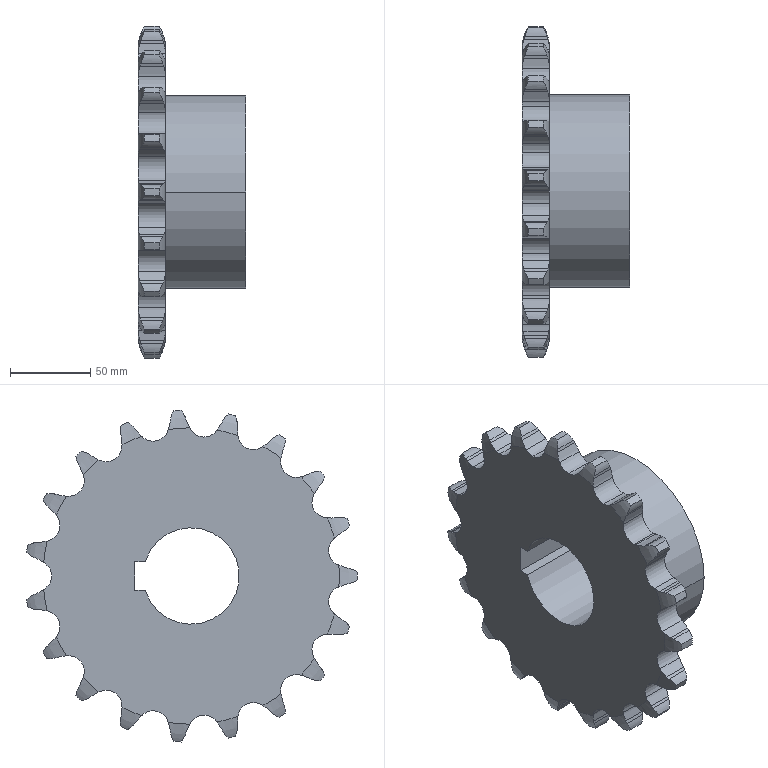Part | STEP file | Produce dryer driving sprocket-1_20A | 1 solid | 208 faces | box 67 x 205.935 x 206.617 mm | volume 832026 mm3 | cylinder 126 | plane 44 | torus 38 | commonest cylinder face diameters 27.844 x40 49.725 x40 19.245 x24 207 x19 120 x2 60 x1